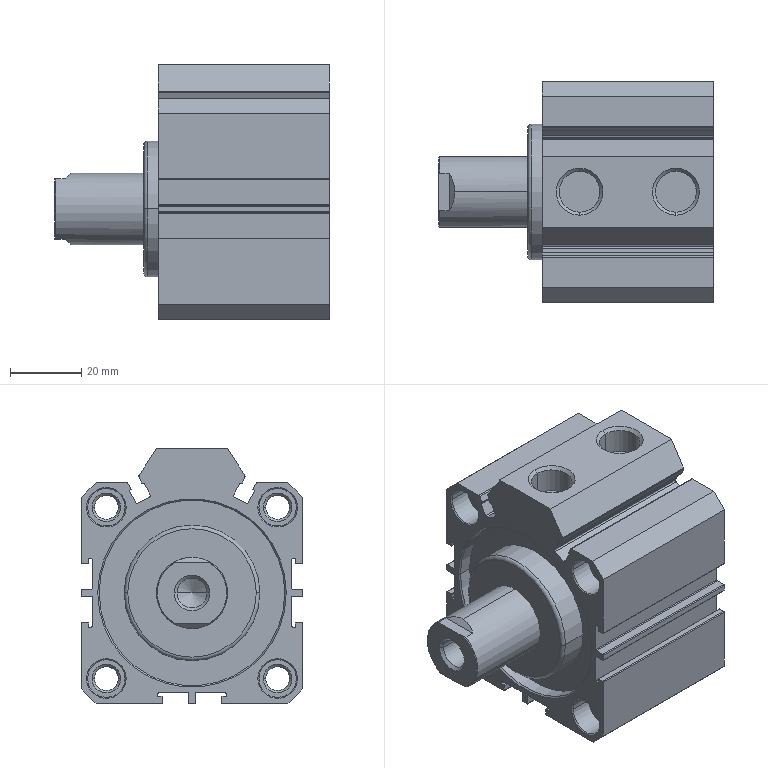Part | SolidWorks | features BaseBody 2, MoveCopyBody 1 | 2 solids | 234 faces | box 77 x 62 x 71.5 mm | volume 138167 mm3 | cylinder 100 | plane 86 | cone 46 | torus 2 | commonest cylinder face diameters 0.4 x46 10.5 x16 0.8 x10 6.647 x8 11.445 x4 20 x4